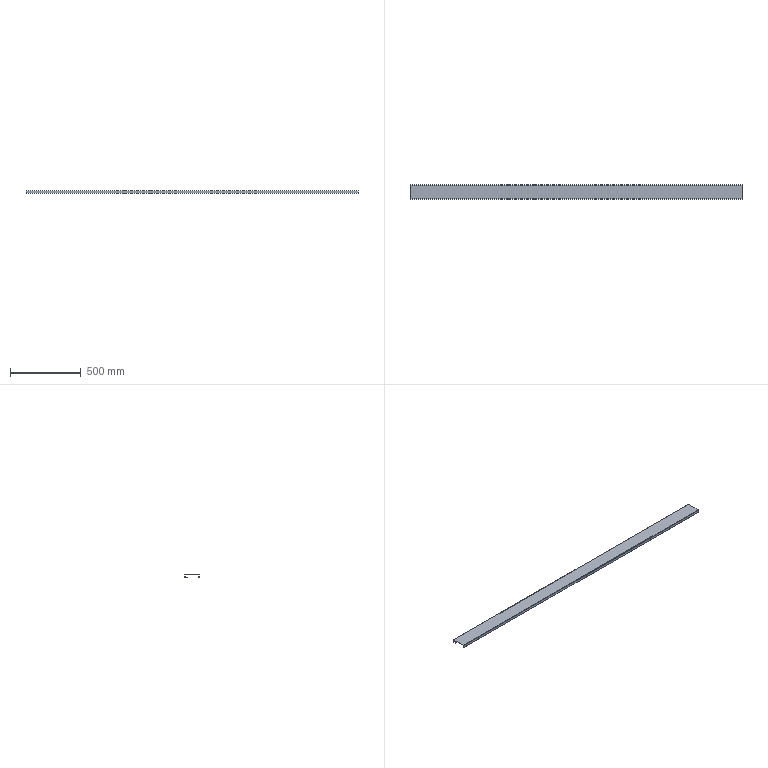Part | STEP file | E3-中转釜护栏8踢脚Plate | 1 solid | 18 faces | box 2340 x 100 x 20 mm | volume 537896 mm3 | plane 12 | cylinder 6 | commonest cylinder face diameters 2 x3 5 x3
STEP:
#1=CARTESIAN_POINT('',(0.,0.,0.));
#2=DIRECTION('',(0.,0.,1.));
#3=DIRECTION('',(1.,0.,0.));
#4=AXIS2_PLACEMENT_3D('',#1,#2,#3);
#5=CARTESIAN_POINT('',(-1170.,1.5,-2.5));
#6=VERTEX_POINT('',#5);
#7=CARTESIAN_POINT('',(-1170.,1.5,-20.));
#8=VERTEX_POINT('',#7);
#9=CARTESIAN_POINT('',(-1170.,1.5,-2.5));
#10=DIRECTION('',(0.,0.,-1.));
#11=VECTOR('',#10,1.);
#12=LINE('',#9,#11);
#13=CARTESIAN_POINT('',(1170.,1.5,-2.5));
#14=DIRECTION('',(0.,-1.,0.));
#15=DIRECTION('',(0.,0.,1.));
#16=AXIS2_PLACEMENT_3D('',#13,#14,#15);
#17=PLANE('',#16);
#18=CARTESIAN_POINT('',(0.,2340.));
#19=DIRECTION('',(-1.,0.));
#20=VECTOR('',#19,1.);
#21=LINE('',#18,#20);
#22=(GEOMETRIC_REPRESENTATION_CONTEXT(2)PARAMETRIC_REPRESENTATION_CONTEXT()REPRESENTATION_CONTEXT('',''));
#23=DEFINITIONAL_REPRESENTATION('',(#21),#22);
#24=PCURVE('',#17,#23);
#25=CARTESIAN_POINT('',(-1170.,2.5,-2.5));
#26=DIRECTION('',(-1.,0.,0.));
#27=DIRECTION('',(0.,0.,-1.));
#28=AXIS2_PLACEMENT_3D('',#25,#26,#27);
#29=PLANE('',#28);
#30=CARTESIAN_POINT('',(0.,1.));
#31=DIRECTION('',(1.,0.));
#32=VECTOR('',#31,1.);
#33=LINE('',#30,#32);
#34=(GEOMETRIC_REPRESENTATION_CONTEXT(2)PARAMETRIC_REPRESENTATION_CONTEXT()REPRESENTATION_CONTEXT('',''));
#35=DEFINITIONAL_REPRESENTATION('',(#33),#34);
#36=PCURVE('',#29,#35);
#37=SURFACE_CURVE('',#12,(#24,#36),.PCURVE_S1.);
#38=EDGE_CURVE('',#6,#8,#37,.T.);
#39=ORIENTED_EDGE('',*,*,#38,.F.);
#40=CARTESIAN_POINT('',(1170.,1.5,-2.5));
#41=VERTEX_POINT('',#40);
#42=CARTESIAN_POINT('',(1170.,1.5,-2.5));
#43=DIRECTION('',(-1.,0.,0.));
#44=VECTOR('',#43,1.);
#45=LINE('',#42,#44);
#46=CARTESIAN_POINT('',(0.,0.));
#47=DIRECTION('',(0.,1.));
#48=VECTOR('',#47,1.);
#49=LINE('',#46,#48);
#50=(GEOMETRIC_REPRESENTATION_CONTEXT(2)PARAMETRIC_REPRESENTATION_CONTEXT()REPRESENTATION_CONTEXT('',''));
#51=DEFINITIONAL_REPRESENTATION('',(#49),#50);
#52=PCURVE('',#17,#51);
#53=CARTESIAN_POINT('',(1170.,2.5,-2.5));
#54=DIRECTION('',(-1.,0.,0.));
#55=DIRECTION('',(0.,0.,-1.));
#56=AXIS2_PLACEMENT_3D('',#53,#54,#55);
#57=CYLINDRICAL_SURFACE('',#56,1.);
#58=CARTESIAN_POINT('',(1.571,0.));
#59=DIRECTION('',(0.,1.));
#60=VECTOR('',#59,1.);
#61=LINE('',#58,#60);
#62=(GEOMETRIC_REPRESENTATION_CONTEXT(2)PARAMETRIC_REPRESENTATION_CONTEXT()REPRESENTATION_CONTEXT('',''));
#63=DEFINITIONAL_REPRESENTATION('',(#61),#62);
#64=PCURVE('',#57,#63);
#65=SURFACE_CURVE('',#45,(#52,#64),.PCURVE_S1.);
#66=EDGE_CURVE('',#41,#6,#65,.T.);
#67=ORIENTED_EDGE('',*,*,#66,.F.);
#68=CARTESIAN_POINT('',(1170.,1.5,-20.));
#69=VERTEX_POINT('',#68);
#70=CARTESIAN_POINT('',(1170.,1.5,-2.5));
#71=DIRECTION('',(0.,0.,-1.));
#72=VECTOR('',#71,1.);
#73=LINE('',#70,#72);
#74=CARTESIAN_POINT('',(0.,0.));
#75=DIRECTION('',(-1.,0.));
#76=VECTOR('',#75,1.);
#77=LINE('',#74,#76);
#78=(GEOMETRIC_REPRESENTATION_CONTEXT(2)PARAMETRIC_REPRESENTATION_CONTEXT()REPRESENTATION_CONTEXT('',''));
#79=DEFINITIONAL_REPRESENTATION('',(#77),#78);
#80=PCURVE('',#17,#79);
#81=CARTESIAN_POINT('',(1170.,2.5,-2.5));
#82=DIRECTION('',(-1.,0.,0.));
#83=DIRECTION('',(0.,0.,-1.));
#84=AXIS2_PLACEMENT_3D('',#81,#82,#83);
#85=PLANE('',#84);
#86=CARTESIAN_POINT('',(0.,1.));
#87=DIRECTION('',(1.,0.));
#88=VECTOR('',#87,1.);
#89=LINE('',#86,#88);
#90=(GEOMETRIC_REPRESENTATION_CONTEXT(2)PARAMETRIC_REPRESENTATION_CONTEXT()REPRESENTATION_CONTEXT('',''));
#91=DEFINITIONAL_REPRESENTATION('',(#89),#90);
#92=PCURVE('',#85,#91);
#93=SURFACE_CURVE('',#73,(#80,#92),.PCURVE_S1.);
#94=EDGE_CURVE('',#41,#69,#93,.T.);
#95=ORIENTED_EDGE('',*,*,#94,.T.);
#96=CARTESIAN_POINT('',(1170.,1.5,-20.));
#97=DIRECTION('',(-1.,0.,0.));
#98=VECTOR('',#97,1.);
#99=LINE('',#96,#98);
#100=CARTESIAN_POINT('',(-17.5,0.));
#101=DIRECTION('',(0.,1.));
#102=VECTOR('',#101,1.);
#103=LINE('',#100,#102);
#104=(GEOMETRIC_REPRESENTATION_CONTEXT(2)PARAMETRIC_REPRESENTATION_CONTEXT()REPRESENTATION_CONTEXT('',''));
#105=DEFINITIONAL_REPRESENTATION('',(#103),#104);
#106=PCURVE('',#17,#105);
#107=CARTESIAN_POINT('',(1170.,0.,-20.));
#108=DIRECTION('',(0.,0.,-1.));
#109=DIRECTION('',(1.,0.,0.));
#110=AXIS2_PLACEMENT_3D('',#107,#108,#109);
#111=PLANE('',#110);
#112=CARTESIAN_POINT('',(0.,-1.5));
#113=DIRECTION('',(-1.,0.));
#114=VECTOR('',#113,1.);
#115=LINE('',#112,#114);
#116=(GEOMETRIC_REPRESENTATION_CONTEXT(2)PARAMETRIC_REPRESENTATION_CONTEXT()REPRESENTATION_CONTEXT('',''));
#117=DEFINITIONAL_REPRESENTATION('',(#115),#116);
#118=PCURVE('',#111,#117);
#119=SURFACE_CURVE('',#99,(#106,#118),.PCURVE_S1.);
#120=EDGE_CURVE('',#69,#8,#119,.T.);
#121=ORIENTED_EDGE('',*,*,#120,.T.);
#122=EDGE_LOOP('',(#39,#67,#95,#121));
#123=FACE_BOUND('',#122,.T.);
#124=ADVANCED_FACE('',(#123),#17,.F.);
#125=CARTESIAN_POINT('',(-1170.,0.,-20.));
#126=VERTEX_POINT('',#125);
#127=CARTESIAN_POINT('',(-1170.,0.,-20.));
#128=DIRECTION('',(0.,1.,0.));
#129=VECTOR('',#128,1.);
#130=LINE('',#127,#129);
#131=CARTESIAN_POINT('',(-2340.,0.));
#132=DIRECTION('',(0.,-1.));
#133=VECTOR('',#132,1.);
#134=LINE('',#131,#133);
#135=(GEOMETRIC_REPRESENTATION_CONTEXT(2)PARAMETRIC_REPRESENTATION_CONTEXT()REPRESENTATION_CONTEXT('',''));
#136=DEFINITIONAL_REPRESENTATION('',(#134),#135);
#137=PCURVE('',#111,#136);
#138=CARTESIAN_POINT('',(17.5,2.5));
#139=DIRECTION('',(0.,-1.));
#140=VECTOR('',#139,1.);
#141=LINE('',#138,#140);
#142=(GEOMETRIC_REPRESENTATION_CONTEXT(2)PARAMETRIC_REPRESENTATION_CONTEXT()REPRESENTATION_CONTEXT('',''));
#143=DEFINITIONAL_REPRESENTATION('',(#141),#142);
#144=PCURVE('',#29,#143);
#145=SURFACE_CURVE('',#130,(#137,#144),.PCURVE_S1.);
#146=EDGE_CURVE('',#126,#8,#145,.T.);
#147=ORIENTED_EDGE('',*,*,#146,.T.);
#148=ORIENTED_EDGE('',*,*,#120,.F.);
#149=CARTESIAN_POINT('',(1170.,0.,-20.));
#150=VERTEX_POINT('',#149);
#151=CARTESIAN_POINT('',(1170.,0.,-20.));
#152=DIRECTION('',(0.,1.,0.));
#153=VECTOR('',#152,1.);
#154=LINE('',#151,#153);
#155=CARTESIAN_POINT('',(0.,0.));
#156=DIRECTION('',(0.,-1.));
#157=VECTOR('',#156,1.);
#158=LINE('',#155,#157);
#159=(GEOMETRIC_REPRESENTATION_CONTEXT(2)PARAMETRIC_REPRESENTATION_CONTEXT()REPRESENTATION_CONTEXT('',''));
#160=DEFINITIONAL_REPRESENTATION('',(#158),#159);
#161=PCURVE('',#111,#160);
#162=CARTESIAN_POINT('',(17.5,2.5));
#163=DIRECTION('',(0.,-1.));
#164=VECTOR('',#163,1.);
#165=LINE('',#162,#164);
#166=(GEOMETRIC_REPRESENTATION_CONTEXT(2)PARAMETRIC_REPRESENTATION_CONTEXT()REPRESENTATION_CONTEXT('',''));
#167=DEFINITIONAL_REPRESENTATION('',(#165),#166);
#168=PCURVE('',#85,#167);
#169=SURFACE_CURVE('',#154,(#161,#168),.PCURVE_S1.);
#170=EDGE_CURVE('',#150,#69,#169,.T.);
#171=ORIENTED_EDGE('',*,*,#170,.F.);
#172=CARTESIAN_POINT('',(1170.,0.,-20.));
#173=DIRECTION('',(-1.,0.,0.));
#174=VECTOR('',#173,1.);
#175=LINE('',#172,#174);
#176=CARTESIAN_POINT('',(0.,0.));
#177=DIRECTION('',(-1.,0.));
#178=VECTOR('',#177,1.);
#179=LINE('',#176,#178);
#180=(GEOMETRIC_REPRESENTATION_CONTEXT(2)PARAMETRIC_REPRESENTATION_CONTEXT()REPRESENTATION_CONTEXT('',''));
#181=DEFINITIONAL_REPRESENTATION('',(#179),#180);
#182=PCURVE('',#111,#181);
#183=CARTESIAN_POINT('',(1170.,0.,-2.5));
#184=DIRECTION('',(0.,-1.,0.));
#185=DIRECTION('',(0.,0.,1.));
#186=AXIS2_PLACEMENT_3D('',#183,#184,#185);
#187=PLANE('',#186);
#188=CARTESIAN_POINT('',(-17.5,0.));
#189=DIRECTION('',(0.,1.));
#190=VECTOR('',#189,1.);
#191=LINE('',#188,#190);
#192=(GEOMETRIC_REPRESENTATION_CONTEXT(2)PARAMETRIC_REPRESENTATION_CONTEXT()REPRESENTATION_CONTEXT('',''));
#193=DEFINITIONAL_REPRESENTATION('',(#191),#192);
#194=PCURVE('',#187,#193);
#195=SURFACE_CURVE('',#175,(#182,#194),.PCURVE_S1.);
#196=EDGE_CURVE('',#150,#126,#195,.T.);
#197=ORIENTED_EDGE('',*,*,#196,.T.);
#198=EDGE_LOOP('',(#147,#148,#171,#197));
#199=FACE_BOUND('',#198,.T.);
#200=ADVANCED_FACE('',(#199),#111,.T.);
#201=CARTESIAN_POINT('',(-1170.,0.,-2.5));
#202=VERTEX_POINT('',#201);
#203=CARTESIAN_POINT('',(-1170.,0.,-2.5));
#204=DIRECTION('',(0.,0.,-1.));
#205=VECTOR('',#204,1.);
#206=LINE('',#203,#205);
#207=CARTESIAN_POINT('',(0.,2340.));
#208=DIRECTION('',(-1.,0.));
#209=VECTOR('',#208,1.);
#210=LINE('',#207,#209);
#211=(GEOMETRIC_REPRESENTATION_CONTEXT(2)PARAMETRIC_REPRESENTATION_CONTEXT()REPRESENTATION_CONTEXT('',''));
#212=DEFINITIONAL_REPRESENTATION('',(#210),#211);
#213=PCURVE('',#187,#212);
#214=CARTESIAN_POINT('',(0.,2.5));
#215=DIRECTION('',(1.,0.));
#216=VECTOR('',#215,1.);
#217=LINE('',#214,#216);
#218=(GEOMETRIC_REPRESENTATION_CONTEXT(2)PARAMETRIC_REPRESENTATION_CONTEXT()REPRESENTATION_CONTEXT('',''));
#219=DEFINITIONAL_REPRESENTATION('',(#217),#218);
#220=PCURVE('',#29,#219);
#221=SURFACE_CURVE('',#206,(#213,#220),.PCURVE_S1.);
#222=EDGE_CURVE('',#202,#126,#221,.T.);
#223=ORIENTED_EDGE('',*,*,#222,.T.);
#224=ORIENTED_EDGE('',*,*,#196,.F.);
#225=CARTESIAN_POINT('',(1170.,0.,-2.5));
#226=VERTEX_POINT('',#225);
#227=CARTESIAN_POINT('',(1170.,0.,-2.5));
#228=DIRECTION('',(0.,0.,-1.));
#229=VECTOR('',#228,1.);
#230=LINE('',#227,#229);
#231=CARTESIAN_POINT('',(0.,0.));
#232=DIRECTION('',(-1.,0.));
#233=VECTOR('',#232,1.);
#234=LINE('',#231,#233);
#235=(GEOMETRIC_REPRESENTATION_CONTEXT(2)PARAMETRIC_REPRESENTATION_CONTEXT()REPRESENTATION_CONTEXT('',''));
#236=DEFINITIONAL_REPRESENTATION('',(#234),#235);
#237=PCURVE('',#187,#236);
#238=CARTESIAN_POINT('',(0.,2.5));
#239=DIRECTION('',(1.,0.));
#240=VECTOR('',#239,1.);
#241=LINE('',#238,#240);
#242=(GEOMETRIC_REPRESENTATION_CONTEXT(2)PARAMETRIC_REPRESENTATION_CONTEXT()REPRESENTATION_CONTEXT('',''));
#243=DEFINITIONAL_REPRESENTATION('',(#241),#242);
#244=PCURVE('',#85,#243);
#245=SURFACE_CURVE('',#230,(#237,#244),.PCURVE_S1.);
#246=EDGE_CURVE('',#226,#150,#245,.T.);
#247=ORIENTED_EDGE('',*,*,#246,.F.);
#248=CARTESIAN_POINT('',(1170.,0.,-2.5));
#249=DIRECTION('',(-1.,0.,0.));
#250=VECTOR('',#249,1.);
#251=LINE('',#248,#250);
#252=CARTESIAN_POINT('',(0.,0.));
#253=DIRECTION('',(0.,1.));
#254=VECTOR('',#253,1.);
#255=LINE('',#252,#254);
#256=(GEOMETRIC_REPRESENTATION_CONTEXT(2)PARAMETRIC_REPRESENTATION_CONTEXT()REPRESENTATION_CONTEXT('',''));
#257=DEFINITIONAL_REPRESENTATION('',(#255),#256);
#258=PCURVE('',#187,#257);
#259=CARTESIAN_POINT('',(1170.,2.5,-2.5));
#260=DIRECTION('',(-1.,0.,0.));
#261=DIRECTION('',(0.,0.,-1.));
#262=AXIS2_PLACEMENT_3D('',#259,#260,#261);
#263=CYLINDRICAL_SURFACE('',#262,2.5);
#264=CARTESIAN_POINT('',(1.571,0.));
#265=DIRECTION('',(0.,1.));
#266=VECTOR('',#265,1.);
#267=LINE('',#264,#266);
#268=(GEOMETRIC_REPRESENTATION_CONTEXT(2)PARAMETRIC_REPRESENTATION_CONTEXT()REPRESENTATION_CONTEXT('',''));
#269=DEFINITIONAL_REPRESENTATION('',(#267),#268);
#270=PCURVE('',#263,#269);
#271=SURFACE_CURVE('',#251,(#258,#270),.PCURVE_S1.);
#272=EDGE_CURVE('',#226,#202,#271,.T.);
#273=ORIENTED_EDGE('',*,*,#272,.T.);
#274=EDGE_LOOP('',(#223,#224,#247,#273));
#275=FACE_BOUND('',#274,.T.);
#276=ADVANCED_FACE('',(#275),#187,.T.);
#277=CARTESIAN_POINT('',(-1170.,2.5,0.));
#278=VERTEX_POINT('',#277);
#279=CARTESIAN_POINT('',(-1170.,2.5,-2.5));
#280=DIRECTION('',(1.,0.,0.));
#281=DIRECTION('',(0.,0.,-1.));
#282=AXIS2_PLACEMENT_3D('',#279,#280,#281);
#283=CIRCLE('',#282,2.5);
#284=CARTESIAN_POINT('',(6.283,2340.));
#285=DIRECTION('',(-1.,0.));
#286=VECTOR('',#285,1.);
#287=LINE('',#284,#286);
#288=(GEOMETRIC_REPRESENTATION_CONTEXT(2)PARAMETRIC_REPRESENTATION_CONTEXT()REPRESENTATION_CONTEXT('',''));
#289=DEFINITIONAL_REPRESENTATION('',(#287),#288);
#290=PCURVE('',#263,#289);
#291=CARTESIAN_POINT('',(2.5,0.));
#292=CARTESIAN_POINT('',(2.5,-4.33));
#293=CARTESIAN_POINT('',(-1.25,-2.165));
#294=CARTESIAN_POINT('',(-5.,0.));
#295=CARTESIAN_POINT('',(-1.25,2.165));
#296=CARTESIAN_POINT('',(2.5,4.33));
#297=CARTESIAN_POINT('',(2.5,0.));
#298=(BOUNDED_CURVE()B_SPLINE_CURVE(2,(#291,#292,#293,#294,#295,#296,#297),.UNSPECIFIED.,.T.,.F.)B_SPLINE_CURVE_WITH_KNOTS((1,2,2,2,2,1),(-2.094,0.,2.094,4.189,6.283,8.378),.UNSPECIFIED.)CURVE()GEOMETRIC_REPRESENTATION_ITEM()RATIONAL_B_SPLINE_CURVE((1.,0.5,1.,0.5,1.,0.5,1.))REPRESENTATION_ITEM(''));
#299=(GEOMETRIC_REPRESENTATION_CONTEXT(2)PARAMETRIC_REPRESENTATION_CONTEXT()REPRESENTATION_CONTEXT('',''));
#300=DEFINITIONAL_REPRESENTATION('',(#298),#299);
#301=PCURVE('',#29,#300);
#302=SURFACE_CURVE('',#283,(#290,#301),.PCURVE_S1.);
#303=EDGE_CURVE('',#278,#202,#302,.T.);
#304=ORIENTED_EDGE('',*,*,#303,.T.);
#305=ORIENTED_EDGE('',*,*,#272,.F.);
#306=CARTESIAN_POINT('',(1170.,2.5,0.));
#307=VERTEX_POINT('',#306);
#308=CARTESIAN_POINT('',(1170.,2.5,-2.5));
#309=DIRECTION('',(1.,0.,0.));
#310=DIRECTION('',(0.,0.,-1.));
#311=AXIS2_PLACEMENT_3D('',#308,#309,#310);
#312=CIRCLE('',#311,2.5);
#313=CARTESIAN_POINT('',(6.283,0.));
#314=DIRECTION('',(-1.,0.));
#315=VECTOR('',#314,1.);
#316=LINE('',#313,#315);
#317=(GEOMETRIC_REPRESENTATION_CONTEXT(2)PARAMETRIC_REPRESENTATION_CONTEXT()REPRESENTATION_CONTEXT('',''));
#318=DEFINITIONAL_REPRESENTATION('',(#316),#317);
#319=PCURVE('',#263,#318);
#320=CARTESIAN_POINT('',(2.5,0.));
#321=CARTESIAN_POINT('',(2.5,-4.33));
#322=CARTESIAN_POINT('',(-1.25,-2.165));
#323=CARTESIAN_POINT('',(-5.,0.));
#324=CARTESIAN_POINT('',(-1.25,2.165));
#325=CARTESIAN_POINT('',(2.5,4.33));
#326=CARTESIAN_POINT('',(2.5,0.));
#327=(BOUNDED_CURVE()B_SPLINE_CURVE(2,(#320,#321,#322,#323,#324,#325,#326),.UNSPECIFIED.,.T.,.F.)B_SPLINE_CURVE_WITH_KNOTS((1,2,2,2,2,1),(-2.094,0.,2.094,4.189,6.283,8.378),.UNSPECIFIED.)CURVE()GEOMETRIC_REPRESENTATION_ITEM()RATIONAL_B_SPLINE_CURVE((1.,0.5,1.,0.5,1.,0.5,1.))REPRESENTATION_ITEM(''));
#328=(GEOMETRIC_REPRESENTATION_CONTEXT(2)PARAMETRIC_REPRESENTATION_CONTEXT()REPRESENTATION_CONTEXT('',''));
#329=DEFINITIONAL_REPRESENTATION('',(#327),#328);
#330=PCURVE('',#85,#329);
#331=SURFACE_CURVE('',#312,(#319,#330),.PCURVE_S1.);
#332=EDGE_CURVE('',#307,#226,#331,.T.);
#333=ORIENTED_EDGE('',*,*,#332,.F.);
#334=CARTESIAN_POINT('',(1170.,2.5,0.));
#335=DIRECTION('',(-1.,0.,0.));
#336=VECTOR('',#335,1.);
#337=LINE('',#334,#336);
#338=CARTESIAN_POINT('',(3.142,0.));
#339=DIRECTION('',(0.,1.));
#340=VECTOR('',#339,1.);
#341=LINE('',#338,#340);
#342=(GEOMETRIC_REPRESENTATION_CONTEXT(2)PARAMETRIC_REPRESENTATION_CONTEXT()REPRESENTATION_CONTEXT('',''));
#343=DEFINITIONAL_REPRESENTATION('',(#341),#342);
#344=PCURVE('',#263,#343);
#345=CARTESIAN_POINT('',(1170.,2.5,0.));
#346=DIRECTION('',(0.,0.,1.));
#347=DIRECTION('',(-1.,0.,0.));
#348=AXIS2_PLACEMENT_3D('',#345,#346,#347);
#349=PLANE('',#348);
#350=CARTESIAN_POINT('',(0.,0.));
#351=DIRECTION('',(1.,0.));
#352=VECTOR('',#351,1.);
#353=LINE('',#350,#352);
#354=(GEOMETRIC_REPRESENTATION_CONTEXT(2)PARAMETRIC_REPRESENTATION_CONTEXT()REPRESENTATION_CONTEXT('',''));
#355=DEFINITIONAL_REPRESENTATION('',(#353),#354);
#356=PCURVE('',#349,#355);
#357=SURFACE_CURVE('',#337,(#344,#356),.PCURVE_S1.);
#358=EDGE_CURVE('',#307,#278,#357,.T.);
#359=ORIENTED_EDGE('',*,*,#358,.T.);
#360=EDGE_LOOP('',(#304,#305,#333,#359));
#361=FACE_BOUND('',#360,.T.);
#362=ADVANCED_FACE('',(#361),#263,.T.);
#363=CARTESIAN_POINT('',(-1170.,97.5,0.));
#364=VERTEX_POINT('',#363);
#365=CARTESIAN_POINT('',(-1170.,2.5,0.));
#366=DIRECTION('',(0.,-1.,0.));
#367=VECTOR('',#366,1.);
#368=LINE('',#365,#367);
#369=CARTESIAN_POINT('',(2340.,0.));
#370=DIRECTION('',(0.,1.));
#371=VECTOR('',#370,1.);
#372=LINE('',#369,#371);
#373=(GEOMETRIC_REPRESENTATION_CONTEXT(2)PARAMETRIC_REPRESENTATION_CONTEXT()REPRESENTATION_CONTEXT('',''));
#374=DEFINITIONAL_REPRESENTATION('',(#372),#373);
#375=PCURVE('',#349,#374);
#376=CARTESIAN_POINT('',(-2.5,0.));
#377=DIRECTION('',(0.,1.));
#378=VECTOR('',#377,1.);
#379=LINE('',#376,#378);
#380=(GEOMETRIC_REPRESENTATION_CONTEXT(2)PARAMETRIC_REPRESENTATION_CONTEXT()REPRESENTATION_CONTEXT('',''));
#381=DEFINITIONAL_REPRESENTATION('',(#379),#380);
#382=PCURVE('',#29,#381);
#383=SURFACE_CURVE('',#368,(#375,#382),.PCURVE_S1.);
#384=EDGE_CURVE('',#364,#278,#383,.T.);
#385=ORIENTED_EDGE('',*,*,#384,.T.);
#386=ORIENTED_EDGE('',*,*,#358,.F.);
#387=CARTESIAN_POINT('',(1170.,97.5,0.));
#388=VERTEX_POINT('',#387);
#389=CARTESIAN_POINT('',(1170.,2.5,0.));
#390=DIRECTION('',(0.,-1.,0.));
#391=VECTOR('',#390,1.);
#392=LINE('',#389,#391);
#393=CARTESIAN_POINT('',(0.,0.));
#394=DIRECTION('',(0.,1.));
#395=VECTOR('',#394,1.);
#396=LINE('',#393,#395);
#397=(GEOMETRIC_REPRESENTATION_CONTEXT(2)PARAMETRIC_REPRESENTATION_CONTEXT()REPRESENTATION_CONTEXT('',''));
#398=DEFINITIONAL_REPRESENTATION('',(#396),#397);
#399=PCURVE('',#349,#398);
#400=CARTESIAN_POINT('',(-2.5,0.));
#401=DIRECTION('',(0.,1.));
#402=VECTOR('',#401,1.);
#403=LINE('',#400,#402);
#404=(GEOMETRIC_REPRESENTATION_CONTEXT(2)PARAMETRIC_REPRESENTATION_CONTEXT()REPRESENTATION_CONTEXT('',''));
#405=DEFINITIONAL_REPRESENTATION('',(#403),#404);
#406=PCURVE('',#85,#405);
#407=SURFACE_CURVE('',#392,(#399,#406),.PCURVE_S1.);
#408=EDGE_CURVE('',#388,#307,#407,.T.);
#409=ORIENTED_EDGE('',*,*,#408,.F.);
#410=CARTESIAN_POINT('',(1170.,97.5,0.));
#411=DIRECTION('',(-1.,0.,0.));
#412=VECTOR('',#411,1.);
#413=LINE('',#410,#412);
#414=CARTESIAN_POINT('',(0.,-95.));
#415=DIRECTION('',(1.,0.));
#416=VECTOR('',#415,1.);
#417=LINE('',#414,#416);
#418=(GEOMETRIC_REPRESENTATION_CONTEXT(2)PARAMETRIC_REPRESENTATION_CONTEXT()REPRESENTATION_CONTEXT('',''));
#419=DEFINITIONAL_REPRESENTATION('',(#417),#418);
#420=PCURVE('',#349,#419);
#421=CARTESIAN_POINT('',(1170.,97.5,-2.5));
#422=DIRECTION('',(-1.,0.,0.));
#423=DIRECTION('',(0.,0.,-1.));
#424=AXIS2_PLACEMENT_3D('',#421,#422,#423);
#425=CYLINDRICAL_SURFACE('',#424,2.5);
#426=CARTESIAN_POINT('',(3.142,0.));
#427=DIRECTION('',(0.,1.));
#428=VECTOR('',#427,1.);
#429=LINE('',#426,#428);
#430=(GEOMETRIC_REPRESENTATION_CONTEXT(2)PARAMETRIC_REPRESENTATION_CONTEXT()REPRESENTATION_CONTEXT('',''));
#431=DEFINITIONAL_REPRESENTATION('',(#429),#430);
#432=PCURVE('',#425,#431);
#433=SURFACE_CURVE('',#413,(#420,#432),.PCURVE_S1.);
#434=EDGE_CURVE('',#388,#364,#433,.T.);
#435=ORIENTED_EDGE('',*,*,#434,.T.);
#436=EDGE_LOOP('',(#385,#386,#409,#435));
#437=FACE_BOUND('',#436,.T.);
#438=ADVANCED_FACE('',(#437),#349,.T.);
#439=CARTESIAN_POINT('',(-1170.,100.,-2.5));
#440=VERTEX_POINT('',#439);
#441=CARTESIAN_POINT('',(-1170.,97.5,-2.5));
#442=DIRECTION('',(1.,0.,0.));
#443=DIRECTION('',(0.,0.,1.));
#444=AXIS2_PLACEMENT_3D('',#441,#442,#443);
#445=CIRCLE('',#444,2.5);
#446=CARTESIAN_POINT('',(9.425,2340.));
#447=DIRECTION('',(-1.,0.));
#448=VECTOR('',#447,1.);
#449=LINE('',#446,#448);
#450=(GEOMETRIC_REPRESENTATION_CONTEXT(2)PARAMETRIC_REPRESENTATION_CONTEXT()REPRESENTATION_CONTEXT('',''));
#451=DEFINITIONAL_REPRESENTATION('',(#449),#450);
#452=PCURVE('',#425,#451);
#453=CARTESIAN_POINT('',(-2.5,-95.));
#454=CARTESIAN_POINT('',(-2.5,-90.67));
#455=CARTESIAN_POINT('',(1.25,-92.835));
#456=CARTESIAN_POINT('',(5.,-95.));
#457=CARTESIAN_POINT('',(1.25,-97.165));
#458=CARTESIAN_POINT('',(-2.5,-99.33));
#459=CARTESIAN_POINT('',(-2.5,-95.));
#460=(BOUNDED_CURVE()B_SPLINE_CURVE(2,(#453,#454,#455,#456,#457,#458,#459),.UNSPECIFIED.,.T.,.F.)B_SPLINE_CURVE_WITH_KNOTS((1,2,2,2,2,1),(-2.094,0.,2.094,4.189,6.283,8.378),.UNSPECIFIED.)CURVE()GEOMETRIC_REPRESENTATION_ITEM()RATIONAL_B_SPLINE_CURVE((1.,0.5,1.,0.5,1.,0.5,1.))REPRESENTATION_ITEM(''));
#461=(GEOMETRIC_REPRESENTATION_CONTEXT(2)PARAMETRIC_REPRESENTATION_CONTEXT()REPRESENTATION_CONTEXT('',''));
#462=DEFINITIONAL_REPRESENTATION('',(#460),#461);
#463=PCURVE('',#29,#462);
#464=SURFACE_CURVE('',#445,(#452,#463),.PCURVE_S1.);
#465=EDGE_CURVE('',#440,#364,#464,.T.);
#466=ORIENTED_EDGE('',*,*,#465,.T.);
#467=ORIENTED_EDGE('',*,*,#434,.F.);
#468=CARTESIAN_POINT('',(1170.,100.,-2.5));
#469=VERTEX_POINT('',#468);
#470=CARTESIAN_POINT('',(1170.,97.5,-2.5));
#471=DIRECTION('',(1.,0.,0.));
#472=DIRECTION('',(0.,0.,1.));
#473=AXIS2_PLACEMENT_3D('',#470,#471,#472);
#474=CIRCLE('',#473,2.5);
#475=CARTESIAN_POINT('',(9.425,0.));
#476=DIRECTION('',(-1.,0.));
#477=VECTOR('',#476,1.);
#478=LINE('',#475,#477);
#479=(GEOMETRIC_REPRESENTATION_CONTEXT(2)PARAMETRIC_REPRESENTATION_CONTEXT()REPRESENTATION_CONTEXT('',''));
#480=DEFINITIONAL_REPRESENTATION('',(#478),#479);
#481=PCURVE('',#425,#480);
#482=CARTESIAN_POINT('',(-2.5,-95.));
#483=CARTESIAN_POINT('',(-2.5,-90.67));
#484=CARTESIAN_POINT('',(1.25,-92.835));
#485=CARTESIAN_POINT('',(5.,-95.));
#486=CARTESIAN_POINT('',(1.25,-97.165));
#487=CARTESIAN_POINT('',(-2.5,-99.33));
#488=CARTESIAN_POINT('',(-2.5,-95.));
#489=(BOUNDED_CURVE()B_SPLINE_CURVE(2,(#482,#483,#484,#485,#486,#487,#488),.UNSPECIFIED.,.T.,.F.)B_SPLINE_CURVE_WITH_KNOTS((1,2,2,2,2,1),(-2.094,0.,2.094,4.189,6.283,8.378),.UNSPECIFIED.)CURVE()GEOMETRIC_REPRESENTATION_ITEM()RATIONAL_B_SPLINE_CURVE((1.,0.5,1.,0.5,1.,0.5,1.))REPRESENTATION_ITEM(''));
#490=(GEOMETRIC_REPRESENTATION_CONTEXT(2)PARAMETRIC_REPRESENTATION_CONTEXT()REPRESENTATION_CONTEXT('',''));
#491=DEFINITIONAL_REPRESENTATION('',(#489),#490);
#492=PCURVE('',#85,#491);
#493=SURFACE_CURVE('',#474,(#481,#492),.PCURVE_S1.);
#494=EDGE_CURVE('',#469,#388,#493,.T.);
#495=ORIENTED_EDGE('',*,*,#494,.F.);
#496=CARTESIAN_POINT('',(1170.,100.,-2.5));
#497=DIRECTION('',(-1.,0.,0.));
#498=VECTOR('',#497,1.);
#499=LINE('',#496,#498);
#500=CARTESIAN_POINT('',(4.712,0.));
#501=DIRECTION('',(0.,1.));
#502=VECTOR('',#501,1.);
#503=LINE('',#500,#502);
#504=(GEOMETRIC_REPRESENTATION_CONTEXT(2)PARAMETRIC_REPRESENTATION_CONTEXT()REPRESENTATION_CONTEXT('',''));
#505=DEFINITIONAL_REPRESENTATION('',(#503),#504);
#506=PCURVE('',#425,#505);
#507=CARTESIAN_POINT('',(1170.,100.,-2.5));
#508=DIRECTION('',(0.,1.,0.));
#509=DIRECTION('',(0.,0.,-1.));
#510=AXIS2_PLACEMENT_3D('',#507,#508,#509);
#511=PLANE('',#510);
#512=CARTESIAN_POINT('',(0.,0.));
#513=DIRECTION('',(0.,1.));
#514=VECTOR('',#513,1.);
#515=LINE('',#512,#514);
#516=(GEOMETRIC_REPRESENTATION_CONTEXT(2)PARAMETRIC_REPRESENTATION_CONTEXT()REPRESENTATION_CONTEXT('',''));
#517=DEFINITIONAL_REPRESENTATION('',(#515),#516);
#518=PCURVE('',#511,#517);
#519=SURFACE_CURVE('',#499,(#506,#518),.PCURVE_S1.);
#520=EDGE_CURVE('',#469,#440,#519,.T.);
#521=ORIENTED_EDGE('',*,*,#520,.T.);
#522=EDGE_LOOP('',(#466,#467,#495,#521));
#523=FACE_BOUND('',#522,.T.);
#524=ADVANCED_FACE('',(#523),#425,.T.);
#525=CARTESIAN_POINT('',(-1170.,100.,-17.5));
#526=VERTEX_POINT('',#525);
#527=CARTESIAN_POINT('',(-1170.,100.,-2.5));
#528=DIRECTION('',(0.,0.,1.));
#529=VECTOR('',#528,1.);
#530=LINE('',#527,#529);
#531=CARTESIAN_POINT('',(0.,2340.));
#532=DIRECTION('',(-1.,0.));
#533=VECTOR('',#532,1.);
#534=LINE('',#531,#533);
#535=(GEOMETRIC_REPRESENTATION_CONTEXT(2)PARAMETRIC_REPRESENTATION_CONTEXT()REPRESENTATION_CONTEXT('',''));
#536=DEFINITIONAL_REPRESENTATION('',(#534),#535);
#537=PCURVE('',#511,#536);
#538=CARTESIAN_POINT('',(0.,-97.5));
#539=DIRECTION('',(-1.,0.));
#540=VECTOR('',#539,1.);
#541=LINE('',#538,#540);
#542=(GEOMETRIC_REPRESENTATION_CONTEXT(2)PARAMETRIC_REPRESENTATION_CONTEXT()REPRESENTATION_CONTEXT('',''));
#543=DEFINITIONAL_REPRESENTATION('',(#541),#542);
#544=PCURVE('',#29,#543);
#545=SURFACE_CURVE('',#530,(#537,#544),.PCURVE_S1.);
#546=EDGE_CURVE('',#526,#440,#545,.T.);
#547=ORIENTED_EDGE('',*,*,#546,.T.);
#548=ORIENTED_EDGE('',*,*,#520,.F.);
#549=CARTESIAN_POINT('',(1170.,100.,-17.5));
#550=VERTEX_POINT('',#549);
#551=CARTESIAN_POINT('',(1170.,100.,-2.5));
#552=DIRECTION('',(0.,0.,1.));
#553=VECTOR('',#552,1.);
#554=LINE('',#551,#553);
#555=CARTESIAN_POINT('',(0.,0.));
#556=DIRECTION('',(-1.,0.));
#557=VECTOR('',#556,1.);
#558=LINE('',#555,#557);
#559=(GEOMETRIC_REPRESENTATION_CONTEXT(2)PARAMETRIC_REPRESENTATION_CONTEXT()REPRESENTATION_CONTEXT('',''));
#560=DEFINITIONAL_REPRESENTATION('',(#558),#559);
#561=PCURVE('',#511,#560);
#562=CARTESIAN_POINT('',(0.,-97.5));
#563=DIRECTION('',(-1.,0.));
#564=VECTOR('',#563,1.);
#565=LINE('',#562,#564);
#566=(GEOMETRIC_REPRESENTATION_CONTEXT(2)PARAMETRIC_REPRESENTATION_CONTEXT()REPRESENTATION_CONTEXT('',''));
#567=DEFINITIONAL_REPRESENTATION('',(#565),#566);
#568=PCURVE('',#85,#567);
#569=SURFACE_CURVE('',#554,(#561,#568),.PCURVE_S1.);
#570=EDGE_CURVE('',#550,#469,#569,.T.);
#571=ORIENTED_EDGE('',*,*,#570,.F.);
#572=CARTESIAN_POINT('',(1170.,100.,-17.5));
#573=DIRECTION('',(-1.,0.,0.));
#574=VECTOR('',#573,1.);
#575=LINE('',#572,#574);
#576=CARTESIAN_POINT('',(15.,0.));
#577=DIRECTION('',(0.,1.));
#578=VECTOR('',#577,1.);
#579=LINE('',#576,#578);
#580=(GEOMETRIC_REPRESENTATION_CONTEXT(2)PARAMETRIC_REPRESENTATION_CONTEXT()REPRESENTATION_CONTEXT('',''));
#581=DEFINITIONAL_REPRESENTATION('',(#579),#580);
#582=PCURVE('',#511,#581);
#583=CARTESIAN_POINT('',(1170.,97.5,-17.5));
#584=DIRECTION('',(-1.,0.,0.));
#585=DIRECTION('',(0.,0.,-1.));
#586=AXIS2_PLACEMENT_3D('',#583,#584,#585);
#587=CYLINDRICAL_SURFACE('',#586,2.5);
#588=CARTESIAN_POINT('',(4.712,0.));
#589=DIRECTION('',(0.,1.));
#590=VECTOR('',#589,1.);
#591=LINE('',#588,#590);
#592=(GEOMETRIC_REPRESENTATION_CONTEXT(2)PARAMETRIC_REPRESENTATION_CONTEXT()REPRESENTATION_CONTEXT('',''));
#593=DEFINITIONAL_REPRESENTATION('',(#591),#592);
#594=PCURVE('',#587,#593);
#595=SURFACE_CURVE('',#575,(#582,#594),.PCURVE_S1.);
#596=EDGE_CURVE('',#550,#526,#595,.T.);
#597=ORIENTED_EDGE('',*,*,#596,.T.);
#598=EDGE_LOOP('',(#547,#548,#571,#597));
#599=FACE_BOUND('',#598,.T.);
#600=ADVANCED_FACE('',(#599),#511,.T.);
#601=CARTESIAN_POINT('',(-1170.,97.5,-20.));
#602=VERTEX_POINT('',#601);
#603=CARTESIAN_POINT('',(-1170.,97.5,-17.5));
#604=DIRECTION('',(1.,0.,0.));
#605=DIRECTION('',(0.,0.,1.));
#606=AXIS2_PLACEMENT_3D('',#603,#604,#605);
#607=CIRCLE('',#606,2.5);
#608=CARTESIAN_POINT('',(9.425,2340.));
#609=DIRECTION('',(-1.,0.));
#610=VECTOR('',#609,1.);
#611=LINE('',#608,#610);
#612=(GEOMETRIC_REPRESENTATION_CONTEXT(2)PARAMETRIC_REPRESENTATION_CONTEXT()REPRESENTATION_CONTEXT('',''));
#613=DEFINITIONAL_REPRESENTATION('',(#611),#612);
#614=PCURVE('',#587,#613);
#615=CARTESIAN_POINT('',(12.5,-95.));
#616=CARTESIAN_POINT('',(12.5,-90.67));
#617=CARTESIAN_POINT('',(16.25,-92.835));
#618=CARTESIAN_POINT('',(20.,-95.));
#619=CARTESIAN_POINT('',(16.25,-97.165));
#620=CARTESIAN_POINT('',(12.5,-99.33));
#621=CARTESIAN_POINT('',(12.5,-95.));
#622=(BOUNDED_CURVE()B_SPLINE_CURVE(2,(#615,#616,#617,#618,#619,#620,#621),.UNSPECIFIED.,.T.,.F.)B_SPLINE_CURVE_WITH_KNOTS((1,2,2,2,2,1),(-2.094,0.,2.094,4.189,6.283,8.378),.UNSPECIFIED.)CURVE()GEOMETRIC_REPRESENTATION_ITEM()RATIONAL_B_SPLINE_CURVE((1.,0.5,1.,0.5,1.,0.5,1.))REPRESENTATION_ITEM(''));
#623=(GEOMETRIC_REPRESENTATION_CONTEXT(2)PARAMETRIC_REPRESENTATION_CONTEXT()REPRESENTATION_CONTEXT('',''));
#624=DEFINITIONAL_REPRESENTATION('',(#622),#623);
#625=PCURVE('',#29,#624);
#626=SURFACE_CURVE('',#607,(#614,#625),.PCURVE_S1.);
#627=EDGE_CURVE('',#602,#526,#626,.T.);
#628=ORIENTED_EDGE('',*,*,#627,.T.);
#629=ORIENTED_EDGE('',*,*,#596,.F.);
#630=CARTESIAN_POINT('',(1170.,97.5,-20.));
#631=VERTEX_POINT('',#630);
#632=CARTESIAN_POINT('',(1170.,97.5,-17.5));
#633=DIRECTION('',(1.,0.,0.));
#634=DIRECTION('',(0.,0.,1.));
#635=AXIS2_PLACEMENT_3D('',#632,#633,#634);
#636=CIRCLE('',#635,2.5);
#637=CARTESIAN_POINT('',(9.425,0.));
#638=DIRECTION('',(-1.,0.));
#639=VECTOR('',#638,1.);
#640=LINE('',#637,#639);
#641=(GEOMETRIC_REPRESENTATION_CONTEXT(2)PARAMETRIC_REPRESENTATION_CONTEXT()REPRESENTATION_CONTEXT('',''));
#642=DEFINITIONAL_REPRESENTATION('',(#640),#641);
#643=PCURVE('',#587,#642);
#644=CARTESIAN_POINT('',(12.5,-95.));
#645=CARTESIAN_POINT('',(12.5,-90.67));
#646=CARTESIAN_POINT('',(16.25,-92.835));
#647=CARTESIAN_POINT('',(20.,-95.));
#648=CARTESIAN_POINT('',(16.25,-97.165));
#649=CARTESIAN_POINT('',(12.5,-99.33));
#650=CARTESIAN_POINT('',(12.5,-95.));
#651=(BOUNDED_CURVE()B_SPLINE_CURVE(2,(#644,#645,#646,#647,#648,#649,#650),.UNSPECIFIED.,.T.,.F.)B_SPLINE_CURVE_WITH_KNOTS((1,2,2,2,2,1),(-2.094,0.,2.094,4.189,6.283,8.378),.UNSPECIFIED.)CURVE()GEOMETRIC_REPRESENTATION_ITEM()RATIONAL_B_SPLINE_CURVE((1.,0.5,1.,0.5,1.,0.5,1.))REPRESENTATION_ITEM(''));
#652=(GEOMETRIC_REPRESENTATION_CONTEXT(2)PARAMETRIC_REPRESENTATION_CONTEXT()REPRESENTATION_CONTEXT('',''));
#653=DEFINITIONAL_REPRESENTATION('',(#651),#652);
#654=PCURVE('',#85,#653);
#655=SURFACE_CURVE('',#636,(#643,#654),.PCURVE_S1.);
#656=EDGE_CURVE('',#631,#550,#655,.T.);
#657=ORIENTED_EDGE('',*,*,#656,.F.);
#658=CARTESIAN_POINT('',(1170.,97.5,-20.));
#659=DIRECTION('',(-1.,0.,0.));
#660=VECTOR('',#659,1.);
#661=LINE('',#658,#660);
#662=CARTESIAN_POINT('',(6.283,0.));
#663=DIRECTION('',(0.,1.));
#664=VECTOR('',#663,1.);
#665=LINE('',#662,#664);
#666=(GEOMETRIC_REPRESENTATION_CONTEXT(2)PARAMETRIC_REPRESENTATION_CONTEXT()REPRESENTATION_CONTEXT('',''));
#667=DEFINITIONAL_REPRESENTATION('',(#665),#666);
#668=PCURVE('',#587,#667);
#669=CARTESIAN_POINT('',(1170.,97.5,-20.));
#670=DIRECTION('',(0.,0.,-1.));
#671=DIRECTION('',(1.,0.,0.));
#672=AXIS2_PLACEMENT_3D('',#669,#670,#671);
#673=PLANE('',#672);
#674=CARTESIAN_POINT('',(0.,0.));
#675=DIRECTION('',(-1.,0.));
#676=VECTOR('',#675,1.);
#677=LINE('',#674,#676);
#678=(GEOMETRIC_REPRESENTATION_CONTEXT(2)PARAMETRIC_REPRESENTATION_CONTEXT()REPRESENTATION_CONTEXT('',''));
#679=DEFINITIONAL_REPRESENTATION('',(#677),#678);
#680=PCURVE('',#673,#679);
#681=SURFACE_CURVE('',#661,(#668,#680),.PCURVE_S1.);
#682=EDGE_CURVE('',#631,#602,#681,.T.);
#683=ORIENTED_EDGE('',*,*,#682,.T.);
#684=EDGE_LOOP('',(#628,#629,#657,#683));
#685=FACE_BOUND('',#684,.T.);
#686=ADVANCED_FACE('',(#685),#587,.T.);
#687=CARTESIAN_POINT('',(-1170.,80.,-20.));
#688=VERTEX_POINT('',#687);
#689=CARTESIAN_POINT('',(-1170.,97.5,-20.));
#690=DIRECTION('',(0.,1.,0.));
#691=VECTOR('',#690,1.);
#692=LINE('',#689,#691);
#693=CARTESIAN_POINT('',(-2340.,0.));
#694=DIRECTION('',(0.,-1.));
#695=VECTOR('',#694,1.);
#696=LINE('',#693,#695);
#697=(GEOMETRIC_REPRESENTATION_CONTEXT(2)PARAMETRIC_REPRESENTATION_CONTEXT()REPRESENTATION_CONTEXT('',''));
#698=DEFINITIONAL_REPRESENTATION('',(#696),#697);
#699=PCURVE('',#673,#698);
#700=CARTESIAN_POINT('',(17.5,-95.));
#701=DIRECTION('',(0.,-1.));
#702=VECTOR('',#701,1.);
#703=LINE('',#700,#702);
#704=(GEOMETRIC_REPRESENTATION_CONTEXT(2)PARAMETRIC_REPRESENTATION_CONTEXT()REPRESENTATION_CONTEXT('',''));
#705=DEFINITIONAL_REPRESENTATION('',(#703),#704);
#706=PCURVE('',#29,#705);
#707=SURFACE_CURVE('',#692,(#699,#706),.PCURVE_S1.);
#708=EDGE_CURVE('',#688,#602,#707,.T.);
#709=ORIENTED_EDGE('',*,*,#708,.T.);
#710=ORIENTED_EDGE('',*,*,#682,.F.);
#711=CARTESIAN_POINT('',(1170.,80.,-20.));
#712=VERTEX_POINT('',#711);
#713=CARTESIAN_POINT('',(1170.,97.5,-20.));
#714=DIRECTION('',(0.,1.,0.));
#715=VECTOR('',#714,1.);
#716=LINE('',#713,#715);
#717=CARTESIAN_POINT('',(0.,0.));
#718=DIRECTION('',(0.,-1.));
#719=VECTOR('',#718,1.);
#720=LINE('',#717,#719);
#721=(GEOMETRIC_REPRESENTATION_CONTEXT(2)PARAMETRIC_REPRESENTATION_CONTEXT()REPRESENTATION_CONTEXT('',''));
#722=DEFINITIONAL_REPRESENTATION('',(#720),#721);
#723=PCURVE('',#673,#722);
#724=CARTESIAN_POINT('',(17.5,-95.));
#725=DIRECTION('',(0.,-1.));
#726=VECTOR('',#725,1.);
#727=LINE('',#724,#726);
#728=(GEOMETRIC_REPRESENTATION_CONTEXT(2)PARAMETRIC_REPRESENTATION_CONTEXT()REPRESENTATION_CONTEXT('',''));
#729=DEFINITIONAL_REPRESENTATION('',(#727),#728);
#730=PCURVE('',#85,#729);
#731=SURFACE_CURVE('',#716,(#723,#730),.PCURVE_S1.);
#732=EDGE_CURVE('',#712,#631,#731,.T.);
#733=ORIENTED_EDGE('',*,*,#732,.F.);
#734=CARTESIAN_POINT('',(1170.,80.,-20.));
#735=DIRECTION('',(-1.,0.,0.));
#736=VECTOR('',#735,1.);
#737=LINE('',#734,#736);
#738=CARTESIAN_POINT('',(0.,17.5));
#739=DIRECTION('',(-1.,0.));
#740=VECTOR('',#739,1.);
#741=LINE('',#738,#740);
#742=(GEOMETRIC_REPRESENTATION_CONTEXT(2)PARAMETRIC_REPRESENTATION_CONTEXT()REPRESENTATION_CONTEXT('',''));
#743=DEFINITIONAL_REPRESENTATION('',(#741),#742);
#744=PCURVE('',#673,#743);
#745=CARTESIAN_POINT('',(1170.,80.,-18.5));
#746=DIRECTION('',(0.,-1.,0.));
#747=DIRECTION('',(0.,0.,1.));
#748=AXIS2_PLACEMENT_3D('',#745,#746,#747);
#749=PLANE('',#748);
#750=CARTESIAN_POINT('',(-1.5,0.));
#751=DIRECTION('',(0.,1.));
#752=VECTOR('',#751,1.);
#753=LINE('',#750,#752);
#754=(GEOMETRIC_REPRESENTATION_CONTEXT(2)PARAMETRIC_REPRESENTATION_CONTEXT()REPRESENTATION_CONTEXT('',''));
#755=DEFINITIONAL_REPRESENTATION('',(#753),#754);
#756=PCURVE('',#749,#755);
#757=SURFACE_CURVE('',#737,(#744,#756),.PCURVE_S1.);
#758=EDGE_CURVE('',#712,#688,#757,.T.);
#759=ORIENTED_EDGE('',*,*,#758,.T.);
#760=EDGE_LOOP('',(#709,#710,#733,#759));
#761=FACE_BOUND('',#760,.T.);
#762=ADVANCED_FACE('',(#761),#673,.T.);
#763=CARTESIAN_POINT('',(-1170.,80.,-18.5));
#764=VERTEX_POINT('',#763);
#765=CARTESIAN_POINT('',(-1170.,80.,-18.5));
#766=DIRECTION('',(0.,0.,-1.));
#767=VECTOR('',#766,1.);
#768=LINE('',#765,#767);
#769=CARTESIAN_POINT('',(0.,2340.));
#770=DIRECTION('',(-1.,0.));
#771=VECTOR('',#770,1.);
#772=LINE('',#769,#771);
#773=(GEOMETRIC_REPRESENTATION_CONTEXT(2)PARAMETRIC_REPRESENTATION_CONTEXT()REPRESENTATION_CONTEXT('',''));
#774=DEFINITIONAL_REPRESENTATION('',(#772),#773);
#775=PCURVE('',#749,#774);
#776=CARTESIAN_POINT('',(16.,-77.5));
#777=DIRECTION('',(1.,0.));
#778=VECTOR('',#777,1.);
#779=LINE('',#776,#778);
#780=(GEOMETRIC_REPRESENTATION_CONTEXT(2)PARAMETRIC_REPRESENTATION_CONTEXT()REPRESENTATION_CONTEXT('',''));
#781=DEFINITIONAL_REPRESENTATION('',(#779),#780);
#782=PCURVE('',#29,#781);
#783=SURFACE_CURVE('',#768,(#775,#782),.PCURVE_S1.);
#784=EDGE_CURVE('',#764,#688,#783,.T.);
#785=ORIENTED_EDGE('',*,*,#784,.T.);
#786=ORIENTED_EDGE('',*,*,#758,.F.);
#787=CARTESIAN_POINT('',(1170.,80.,-18.5));
#788=VERTEX_POINT('',#787);
#789=CARTESIAN_POINT('',(1170.,80.,-18.5));
#790=DIRECTION('',(0.,0.,-1.));
#791=VECTOR('',#790,1.);
#792=LINE('',#789,#791);
#793=CARTESIAN_POINT('',(0.,0.));
#794=DIRECTION('',(-1.,0.));
#795=VECTOR('',#794,1.);
#796=LINE('',#793,#795);
#797=(GEOMETRIC_REPRESENTATION_CONTEXT(2)PARAMETRIC_REPRESENTATION_CONTEXT()REPRESENTATION_CONTEXT('',''));
#798=DEFINITIONAL_REPRESENTATION('',(#796),#797);
#799=PCURVE('',#749,#798);
#800=CARTESIAN_POINT('',(16.,-77.5));
#801=DIRECTION('',(1.,0.));
#802=VECTOR('',#801,1.);
#803=LINE('',#800,#802);
#804=(GEOMETRIC_REPRESENTATION_CONTEXT(2)PARAMETRIC_REPRESENTATION_CONTEXT()REPRESENTATION_CONTEXT('',''));
#805=DEFINITIONAL_REPRESENTATION('',(#803),#804);
#806=PCURVE('',#85,#805);
#807=SURFACE_CURVE('',#792,(#799,#806),.PCURVE_S1.);
#808=EDGE_CURVE('',#788,#712,#807,.T.);
#809=ORIENTED_EDGE('',*,*,#808,.F.);
#810=CARTESIAN_POINT('',(1170.,80.,-18.5));
#811=DIRECTION('',(-1.,0.,0.));
#812=VECTOR('',#811,1.);
#813=LINE('',#810,#812);
#814=CARTESIAN_POINT('',(0.,0.));
#815=DIRECTION('',(0.,1.));
#816=VECTOR('',#815,1.);
#817=LINE('',#814,#816);
#818=(GEOMETRIC_REPRESENTATION_CONTEXT(2)PARAMETRIC_REPRESENTATION_CONTEXT()REPRESENTATION_CONTEXT('',''));
#819=DEFINITIONAL_REPRESENTATION('',(#817),#818);
#820=PCURVE('',#749,#819);
#821=CARTESIAN_POINT('',(1170.,97.5,-18.5));
#822=DIRECTION('',(0.,0.,-1.));
#823=DIRECTION('',(1.,0.,0.));
#824=AXIS2_PLACEMENT_3D('',#821,#822,#823);
#825=PLANE('',#824);
#826=CARTESIAN_POINT('',(0.,17.5));
#827=DIRECTION('',(-1.,0.));
#828=VECTOR('',#827,1.);
#829=LINE('',#826,#828);
#830=(GEOMETRIC_REPRESENTATION_CONTEXT(2)PARAMETRIC_REPRESENTATION_CONTEXT()REPRESENTATION_CONTEXT('',''));
#831=DEFINITIONAL_REPRESENTATION('',(#829),#830);
#832=PCURVE('',#825,#831);
#833=SURFACE_CURVE('',#813,(#820,#832),.PCURVE_S1.);
#834=EDGE_CURVE('',#788,#764,#833,.T.);
#835=ORIENTED_EDGE('',*,*,#834,.T.);
#836=EDGE_LOOP('',(#785,#786,#809,#835));
#837=FACE_BOUND('',#836,.T.);
#838=ADVANCED_FACE('',(#837),#749,.T.);
#839=CARTESIAN_POINT('',(-1170.,97.5,-18.5));
#840=VERTEX_POINT('',#839);
#841=CARTESIAN_POINT('',(-1170.,97.5,-18.5));
#842=DIRECTION('',(0.,1.,0.));
#843=VECTOR('',#842,1.);
#844=LINE('',#841,#843);
#845=CARTESIAN_POINT('',(-2340.,0.));
#846=DIRECTION('',(0.,-1.));
#847=VECTOR('',#846,1.);
#848=LINE('',#845,#847);
#849=(GEOMETRIC_REPRESENTATION_CONTEXT(2)PARAMETRIC_REPRESENTATION_CONTEXT()REPRESENTATION_CONTEXT('',''));
#850=DEFINITIONAL_REPRESENTATION('',(#848),#849);
#851=PCURVE('',#825,#850);
#852=CARTESIAN_POINT('',(16.,-95.));
#853=DIRECTION('',(0.,-1.));
#854=VECTOR('',#853,1.);
#855=LINE('',#852,#854);
#856=(GEOMETRIC_REPRESENTATION_CONTEXT(2)PARAMETRIC_REPRESENTATION_CONTEXT()REPRESENTATION_CONTEXT('',''));
#857=DEFINITIONAL_REPRESENTATION('',(#855),#856);
#858=PCURVE('',#29,#857);
#859=SURFACE_CURVE('',#844,(#851,#858),.PCURVE_S1.);
#860=EDGE_CURVE('',#764,#840,#859,.T.);
#861=ORIENTED_EDGE('',*,*,#860,.F.);
#862=ORIENTED_EDGE('',*,*,#834,.F.);
#863=CARTESIAN_POINT('',(1170.,97.5,-18.5));
#864=VERTEX_POINT('',#863);
#865=CARTESIAN_POINT('',(1170.,97.5,-18.5));
#866=DIRECTION('',(0.,1.,0.));
#867=VECTOR('',#866,1.);
#868=LINE('',#865,#867);
#869=CARTESIAN_POINT('',(0.,0.));
#870=DIRECTION('',(0.,-1.));
#871=VECTOR('',#870,1.);
#872=LINE('',#869,#871);
#873=(GEOMETRIC_REPRESENTATION_CONTEXT(2)PARAMETRIC_REPRESENTATION_CONTEXT()REPRESENTATION_CONTEXT('',''));
#874=DEFINITIONAL_REPRESENTATION('',(#872),#873);
#875=PCURVE('',#825,#874);
#876=CARTESIAN_POINT('',(16.,-95.));
#877=DIRECTION('',(0.,-1.));
#878=VECTOR('',#877,1.);
#879=LINE('',#876,#878);
#880=(GEOMETRIC_REPRESENTATION_CONTEXT(2)PARAMETRIC_REPRESENTATION_CONTEXT()REPRESENTATION_CONTEXT('',''));
#881=DEFINITIONAL_REPRESENTATION('',(#879),#880);
#882=PCURVE('',#85,#881);
#883=SURFACE_CURVE('',#868,(#875,#882),.PCURVE_S1.);
#884=EDGE_CURVE('',#788,#864,#883,.T.);
#885=ORIENTED_EDGE('',*,*,#884,.T.);
#886=CARTESIAN_POINT('',(1170.,97.5,-18.5));
#887=DIRECTION('',(-1.,0.,0.));
#888=VECTOR('',#887,1.);
#889=LINE('',#886,#888);
#890=CARTESIAN_POINT('',(0.,0.));
#891=DIRECTION('',(-1.,0.));
#892=VECTOR('',#891,1.);
#893=LINE('',#890,#892);
#894=(GEOMETRIC_REPRESENTATION_CONTEXT(2)PARAMETRIC_REPRESENTATION_CONTEXT()REPRESENTATION_CONTEXT('',''));
#895=DEFINITIONAL_REPRESENTATION('',(#893),#894);
#896=PCURVE('',#825,#895);
#897=CARTESIAN_POINT('',(1170.,97.5,-17.5));
#898=DIRECTION('',(-1.,0.,0.));
#899=DIRECTION('',(0.,0.,-1.));
#900=AXIS2_PLACEMENT_3D('',#897,#898,#899);
#901=CYLINDRICAL_SURFACE('',#900,1.);
#902=CARTESIAN_POINT('',(6.283,0.));
#903=DIRECTION('',(0.,1.));
#904=VECTOR('',#903,1.);
#905=LINE('',#902,#904);
#906=(GEOMETRIC_REPRESENTATION_CONTEXT(2)PARAMETRIC_REPRESENTATION_CONTEXT()REPRESENTATION_CONTEXT('',''));
#907=DEFINITIONAL_REPRESENTATION('',(#905),#906);
#908=PCURVE('',#901,#907);
#909=SURFACE_CURVE('',#889,(#896,#908),.PCURVE_S1.);
#910=EDGE_CURVE('',#864,#840,#909,.T.);
#911=ORIENTED_EDGE('',*,*,#910,.T.);
#912=EDGE_LOOP('',(#861,#862,#885,#911));
#913=FACE_BOUND('',#912,.T.);
#914=ADVANCED_FACE('',(#913),#825,.F.);
#915=CARTESIAN_POINT('',(1170.,98.5,-17.5));
#916=VERTEX_POINT('',#915);
#917=CARTESIAN_POINT('',(-1170.,98.5,-17.5));
#918=VERTEX_POINT('',#917);
#919=CARTESIAN_POINT('',(1170.,98.5,-17.5));
#920=DIRECTION('',(-1.,0.,0.));
#921=VECTOR('',#920,1.);
#922=LINE('',#919,#921);
#923=CARTESIAN_POINT('',(4.712,0.));
#924=DIRECTION('',(0.,1.));
#925=VECTOR('',#924,1.);
#926=LINE('',#923,#925);
#927=(GEOMETRIC_REPRESENTATION_CONTEXT(2)PARAMETRIC_REPRESENTATION_CONTEXT()REPRESENTATION_CONTEXT('',''));
#928=DEFINITIONAL_REPRESENTATION('',(#926),#927);
#929=PCURVE('',#901,#928);
#930=CARTESIAN_POINT('',(1170.,98.5,-2.5));
#931=DIRECTION('',(0.,1.,0.));
#932=DIRECTION('',(0.,0.,-1.));
#933=AXIS2_PLACEMENT_3D('',#930,#931,#932);
#934=PLANE('',#933);
#935=CARTESIAN_POINT('',(15.,0.));
#936=DIRECTION('',(0.,1.));
#937=VECTOR('',#936,1.);
#938=LINE('',#935,#937);
#939=(GEOMETRIC_REPRESENTATION_CONTEXT(2)PARAMETRIC_REPRESENTATION_CONTEXT()REPRESENTATION_CONTEXT('',''));
#940=DEFINITIONAL_REPRESENTATION('',(#938),#939);
#941=PCURVE('',#934,#940);
#942=SURFACE_CURVE('',#922,(#929,#941),.PCURVE_S1.);
#943=EDGE_CURVE('',#916,#918,#942,.T.);
#944=ORIENTED_EDGE('',*,*,#943,.F.);
#945=CARTESIAN_POINT('',(1170.,97.5,-17.5));
#946=DIRECTION('',(1.,0.,0.));
#947=DIRECTION('',(0.,0.,1.));
#948=AXIS2_PLACEMENT_3D('',#945,#946,#947);
#949=CIRCLE('',#948,1.);
#950=CARTESIAN_POINT('',(9.425,0.));
#951=DIRECTION('',(-1.,0.));
#952=VECTOR('',#951,1.);
#953=LINE('',#950,#952);
#954=(GEOMETRIC_REPRESENTATION_CONTEXT(2)PARAMETRIC_REPRESENTATION_CONTEXT()REPRESENTATION_CONTEXT('',''));
#955=DEFINITIONAL_REPRESENTATION('',(#953),#954);
#956=PCURVE('',#901,#955);
#957=CARTESIAN_POINT('',(14.,-95.));
#958=CARTESIAN_POINT('',(14.,-93.268));
#959=CARTESIAN_POINT('',(15.5,-94.134));
#960=CARTESIAN_POINT('',(17.,-95.));
#961=CARTESIAN_POINT('',(15.5,-95.866));
#962=CARTESIAN_POINT('',(14.,-96.732));
#963=CARTESIAN_POINT('',(14.,-95.));
#964=(BOUNDED_CURVE()B_SPLINE_CURVE(2,(#957,#958,#959,#960,#961,#962,#963),.UNSPECIFIED.,.T.,.F.)B_SPLINE_CURVE_WITH_KNOTS((1,2,2,2,2,1),(-2.094,0.,2.094,4.189,6.283,8.378),.UNSPECIFIED.)CURVE()GEOMETRIC_REPRESENTATION_ITEM()RATIONAL_B_SPLINE_CURVE((1.,0.5,1.,0.5,1.,0.5,1.))REPRESENTATION_ITEM(''));
#965=(GEOMETRIC_REPRESENTATION_CONTEXT(2)PARAMETRIC_REPRESENTATION_CONTEXT()REPRESENTATION_CONTEXT('',''));
#966=DEFINITIONAL_REPRESENTATION('',(#964),#965);
#967=PCURVE('',#85,#966);
#968=SURFACE_CURVE('',#949,(#956,#967),.PCURVE_S1.);
#969=EDGE_CURVE('',#864,#916,#968,.T.);
#970=ORIENTED_EDGE('',*,*,#969,.F.);
#971=ORIENTED_EDGE('',*,*,#910,.T.);
#972=CARTESIAN_POINT('',(-1170.,97.5,-17.5));
#973=DIRECTION('',(1.,0.,0.));
#974=DIRECTION('',(0.,0.,1.));
#975=AXIS2_PLACEMENT_3D('',#972,#973,#974);
#976=CIRCLE('',#975,1.);
#977=CARTESIAN_POINT('',(9.425,2340.));
#978=DIRECTION('',(-1.,0.));
#979=VECTOR('',#978,1.);
#980=LINE('',#977,#979);
#981=(GEOMETRIC_REPRESENTATION_CONTEXT(2)PARAMETRIC_REPRESENTATION_CONTEXT()REPRESENTATION_CONTEXT('',''));
#982=DEFINITIONAL_REPRESENTATION('',(#980),#981);
#983=PCURVE('',#901,#982);
#984=CARTESIAN_POINT('',(14.,-95.));
#985=CARTESIAN_POINT('',(14.,-93.268));
#986=CARTESIAN_POINT('',(15.5,-94.134));
#987=CARTESIAN_POINT('',(17.,-95.));
#988=CARTESIAN_POINT('',(15.5,-95.866));
#989=CARTESIAN_POINT('',(14.,-96.732));
#990=CARTESIAN_POINT('',(14.,-95.));
#991=(BOUNDED_CURVE()B_SPLINE_CURVE(2,(#984,#985,#986,#987,#988,#989,#990),.UNSPECIFIED.,.T.,.F.)B_SPLINE_CURVE_WITH_KNOTS((1,2,2,2,2,1),(-2.094,0.,2.094,4.189,6.283,8.378),.UNSPECIFIED.)CURVE()GEOMETRIC_REPRESENTATION_ITEM()RATIONAL_B_SPLINE_CURVE((1.,0.5,1.,0.5,1.,0.5,1.))REPRESENTATION_ITEM(''));
#992=(GEOMETRIC_REPRESENTATION_CONTEXT(2)PARAMETRIC_REPRESENTATION_CONTEXT()REPRESENTATION_CONTEXT('',''));
#993=DEFINITIONAL_REPRESENTATION('',(#991),#992);
#994=PCURVE('',#29,#993);
#995=SURFACE_CURVE('',#976,(#983,#994),.PCURVE_S1.);
#996=EDGE_CURVE('',#840,#918,#995,.T.);
#997=ORIENTED_EDGE('',*,*,#996,.T.);
#998=EDGE_LOOP('',(#944,#970,#971,#997));
#999=FACE_BOUND('',#998,.F.);
#1000=ADVANCED_FACE('',(#999),#901,.F.);
#1001=CARTESIAN_POINT('',(-1170.,98.5,-2.5));
#1002=VERTEX_POINT('',#1001);
#1003=CARTESIAN_POINT('',(-1170.,98.5,-2.5));
#1004=DIRECTION('',(0.,0.,1.));
#1005=VECTOR('',#1004,1.);
#1006=LINE('',#1003,#1005);
#1007=CARTESIAN_POINT('',(0.,2340.));
#1008=DIRECTION('',(-1.,0.));
#1009=VECTOR('',#1008,1.);
#1010=LINE('',#1007,#1009);
#1011=(GEOMETRIC_REPRESENTATION_CONTEXT(2)PARAMETRIC_REPRESENTATION_CONTEXT()REPRESENTATION_CONTEXT('',''));
#1012=DEFINITIONAL_REPRESENTATION('',(#1010),#1011);
#1013=PCURVE('',#934,#1012);
#1014=CARTESIAN_POINT('',(0.,-96.));
#1015=DIRECTION('',(-1.,0.));
#1016=VECTOR('',#1015,1.);
#1017=LINE('',#1014,#1016);
#1018=(GEOMETRIC_REPRESENTATION_CONTEXT(2)PARAMETRIC_REPRESENTATION_CONTEXT()REPRESENTATION_CONTEXT('',''));
#1019=DEFINITIONAL_REPRESENTATION('',(#1017),#1018);
#1020=PCURVE('',#29,#1019);
#1021=SURFACE_CURVE('',#1006,(#1013,#1020),.PCURVE_S1.);
#1022=EDGE_CURVE('',#918,#1002,#1021,.T.);
#1023=ORIENTED_EDGE('',*,*,#1022,.F.);
#1024=ORIENTED_EDGE('',*,*,#943,.F.);
#1025=CARTESIAN_POINT('',(1170.,98.5,-2.5));
#1026=VERTEX_POINT('',#1025);
#1027=CARTESIAN_POINT('',(1170.,98.5,-2.5));
#1028=DIRECTION('',(0.,0.,1.));
#1029=VECTOR('',#1028,1.);
#1030=LINE('',#1027,#1029);
#1031=CARTESIAN_POINT('',(0.,0.));
#1032=DIRECTION('',(-1.,0.));
#1033=VECTOR('',#1032,1.);
#1034=LINE('',#1031,#1033);
#1035=(GEOMETRIC_REPRESENTATION_CONTEXT(2)PARAMETRIC_REPRESENTATION_CONTEXT()REPRESENTATION_CONTEXT('',''));
#1036=DEFINITIONAL_REPRESENTATION('',(#1034),#1035);
#1037=PCURVE('',#934,#1036);
#1038=CARTESIAN_POINT('',(0.,-96.));
#1039=DIRECTION('',(-1.,0.));
#1040=VECTOR('',#1039,1.);
#1041=LINE('',#1038,#1040);
#1042=(GEOMETRIC_REPRESENTATION_CONTEXT(2)PARAMETRIC_REPRESENTATION_CONTEXT()REPRESENTATION_CONTEXT('',''));
#1043=DEFINITIONAL_REPRESENTATION('',(#1041),#1042);
#1044=PCURVE('',#85,#1043);
#1045=SURFACE_CURVE('',#1030,(#1037,#1044),.PCURVE_S1.);
#1046=EDGE_CURVE('',#916,#1026,#1045,.T.);
#1047=ORIENTED_EDGE('',*,*,#1046,.T.);
#1048=CARTESIAN_POINT('',(1170.,98.5,-2.5));
#1049=DIRECTION('',(-1.,0.,0.));
#1050=VECTOR('',#1049,1.);
#1051=LINE('',#1048,#1050);
#1052=CARTESIAN_POINT('',(0.,0.));
#1053=DIRECTION('',(0.,1.));
#1054=VECTOR('',#1053,1.);
#1055=LINE('',#1052,#1054);
#1056=(GEOMETRIC_REPRESENTATION_CONTEXT(2)PARAMETRIC_REPRESENTATION_CONTEXT()REPRESENTATION_CONTEXT('',''));
#1057=DEFINITIONAL_REPRESENTATION('',(#1055),#1056);
#1058=PCURVE('',#934,#1057);
#1059=CARTESIAN_POINT('',(1170.,97.5,-2.5));
#1060=DIRECTION('',(-1.,0.,0.));
#1061=DIRECTION('',(0.,0.,-1.));
#1062=AXIS2_PLACEMENT_3D('',#1059,#1060,#1061);
#1063=CYLINDRICAL_SURFACE('',#1062,1.);
#1064=CARTESIAN_POINT('',(4.712,0.));
#1065=DIRECTION('',(0.,1.));
#1066=VECTOR('',#1065,1.);
#1067=LINE('',#1064,#1066);
#1068=(GEOMETRIC_REPRESENTATION_CONTEXT(2)PARAMETRIC_REPRESENTATION_CONTEXT()REPRESENTATION_CONTEXT('',''));
#1069=DEFINITIONAL_REPRESENTATION('',(#1067),#1068);
#1070=PCURVE('',#1063,#1069);
#1071=SURFACE_CURVE('',#1051,(#1058,#1070),.PCURVE_S1.);
#1072=EDGE_CURVE('',#1026,#1002,#1071,.T.);
#1073=ORIENTED_EDGE('',*,*,#1072,.T.);
#1074=EDGE_LOOP('',(#1023,#1024,#1047,#1073));
#1075=FACE_BOUND('',#1074,.T.);
#1076=ADVANCED_FACE('',(#1075),#934,.F.);
#1077=CARTESIAN_POINT('',(1170.,97.5,-1.5));
#1078=VERTEX_POINT('',#1077);
#1079=CARTESIAN_POINT('',(-1170.,97.5,-1.5));
#1080=VERTEX_POINT('',#1079);
#1081=CARTESIAN_POINT('',(1170.,97.5,-1.5));
#1082=DIRECTION('',(-1.,0.,0.));
#1083=VECTOR('',#1082,1.);
#1084=LINE('',#1081,#1083);
#1085=CARTESIAN_POINT('',(3.142,0.));
#1086=DIRECTION('',(0.,1.));
#1087=VECTOR('',#1086,1.);
#1088=LINE('',#1085,#1087);
#1089=(GEOMETRIC_REPRESENTATION_CONTEXT(2)PARAMETRIC_REPRESENTATION_CONTEXT()REPRESENTATION_CONTEXT('',''));
#1090=DEFINITIONAL_REPRESENTATION('',(#1088),#1089);
#1091=PCURVE('',#1063,#1090);
#1092=CARTESIAN_POINT('',(1170.,2.5,-1.5));
#1093=DIRECTION('',(0.,0.,1.));
#1094=DIRECTION('',(-1.,0.,0.));
#1095=AXIS2_PLACEMENT_3D('',#1092,#1093,#1094);
#1096=PLANE('',#1095);
#1097=CARTESIAN_POINT('',(0.,-95.));
#1098=DIRECTION('',(1.,0.));
#1099=VECTOR('',#1098,1.);
#1100=LINE('',#1097,#1099);
#1101=(GEOMETRIC_REPRESENTATION_CONTEXT(2)PARAMETRIC_REPRESENTATION_CONTEXT()REPRESENTATION_CONTEXT('',''));
#1102=DEFINITIONAL_REPRESENTATION('',(#1100),#1101);
#1103=PCURVE('',#1096,#1102);
#1104=SURFACE_CURVE('',#1084,(#1091,#1103),.PCURVE_S1.);
#1105=EDGE_CURVE('',#1078,#1080,#1104,.T.);
#1106=ORIENTED_EDGE('',*,*,#1105,.F.);
#1107=CARTESIAN_POINT('',(1170.,97.5,-2.5));
#1108=DIRECTION('',(1.,0.,0.));
#1109=DIRECTION('',(0.,0.,1.));
#1110=AXIS2_PLACEMENT_3D('',#1107,#1108,#1109);
#1111=CIRCLE('',#1110,1.);
#1112=CARTESIAN_POINT('',(9.425,0.));
#1113=DIRECTION('',(-1.,0.));
#1114=VECTOR('',#1113,1.);
#1115=LINE('',#1112,#1114);
#1116=(GEOMETRIC_REPRESENTATION_CONTEXT(2)PARAMETRIC_REPRESENTATION_CONTEXT()REPRESENTATION_CONTEXT('',''));
#1117=DEFINITIONAL_REPRESENTATION('',(#1115),#1116);
#1118=PCURVE('',#1063,#1117);
#1119=CARTESIAN_POINT('',(-1.,-95.));
#1120=CARTESIAN_POINT('',(-1.,-93.268));
#1121=CARTESIAN_POINT('',(0.5,-94.134));
#1122=CARTESIAN_POINT('',(2.,-95.));
#1123=CARTESIAN_POINT('',(0.5,-95.866));
#1124=CARTESIAN_POINT('',(-1.,-96.732));
#1125=CARTESIAN_POINT('',(-1.,-95.));
#1126=(BOUNDED_CURVE()B_SPLINE_CURVE(2,(#1119,#1120,#1121,#1122,#1123,#1124,#1125),.UNSPECIFIED.,.T.,.F.)B_SPLINE_CURVE_WITH_KNOTS((1,2,2,2,2,1),(-2.094,0.,2.094,4.189,6.283,8.378),.UNSPECIFIED.)CURVE()GEOMETRIC_REPRESENTATION_ITEM()RATIONAL_B_SPLINE_CURVE((1.,0.5,1.,0.5,1.,0.5,1.))REPRESENTATION_ITEM(''));
#1127=(GEOMETRIC_REPRESENTATION_CONTEXT(2)PARAMETRIC_REPRESENTATION_CONTEXT()REPRESENTATION_CONTEXT('',''));
#1128=DEFINITIONAL_REPRESENTATION('',(#1126),#1127);
#1129=PCURVE('',#85,#1128);
#1130=SURFACE_CURVE('',#1111,(#1118,#1129),.PCURVE_S1.);
#1131=EDGE_CURVE('',#1026,#1078,#1130,.T.);
#1132=ORIENTED_EDGE('',*,*,#1131,.F.);
#1133=ORIENTED_EDGE('',*,*,#1072,.T.);
#1134=CARTESIAN_POINT('',(-1170.,97.5,-2.5));
#1135=DIRECTION('',(1.,0.,0.));
#1136=DIRECTION('',(0.,0.,1.));
#1137=AXIS2_PLACEMENT_3D('',#1134,#1135,#1136);
#1138=CIRCLE('',#1137,1.);
#1139=CARTESIAN_POINT('',(9.425,2340.));
#1140=DIRECTION('',(-1.,0.));
#1141=VECTOR('',#1140,1.);
#1142=LINE('',#1139,#1141);
#1143=(GEOMETRIC_REPRESENTATION_CONTEXT(2)PARAMETRIC_REPRESENTATION_CONTEXT()REPRESENTATION_CONTEXT('',''));
#1144=DEFINITIONAL_REPRESENTATION('',(#1142),#1143);
#1145=PCURVE('',#1063,#1144);
#1146=CARTESIAN_POINT('',(-1.,-95.));
#1147=CARTESIAN_POINT('',(-1.,-93.268));
#1148=CARTESIAN_POINT('',(0.5,-94.134));
#1149=CARTESIAN_POINT('',(2.,-95.));
#1150=CARTESIAN_POINT('',(0.5,-95.866));
#1151=CARTESIAN_POINT('',(-1.,-96.732));
#1152=CARTESIAN_POINT('',(-1.,-95.));
#1153=(BOUNDED_CURVE()B_SPLINE_CURVE(2,(#1146,#1147,#1148,#1149,#1150,#1151,#1152),.UNSPECIFIED.,.T.,.F.)B_SPLINE_CURVE_WITH_KNOTS((1,2,2,2,2,1),(-2.094,0.,2.094,4.189,6.283,8.378),.UNSPECIFIED.)CURVE()GEOMETRIC_REPRESENTATION_ITEM()RATIONAL_B_SPLINE_CURVE((1.,0.5,1.,0.5,1.,0.5,1.))REPRESENTATION_ITEM(''));
#1154=(GEOMETRIC_REPRESENTATION_CONTEXT(2)PARAMETRIC_REPRESENTATION_CONTEXT()REPRESENTATION_CONTEXT('',''));
#1155=DEFINITIONAL_REPRESENTATION('',(#1153),#1154);
#1156=PCURVE('',#29,#1155);
#1157=SURFACE_CURVE('',#1138,(#1145,#1156),.PCURVE_S1.);
#1158=EDGE_CURVE('',#1002,#1080,#1157,.T.);
#1159=ORIENTED_EDGE('',*,*,#1158,.T.);
#1160=EDGE_LOOP('',(#1106,#1132,#1133,#1159));
#1161=FACE_BOUND('',#1160,.F.);
#1162=ADVANCED_FACE('',(#1161),#1063,.F.);
#1163=CARTESIAN_POINT('',(-1170.,2.5,-1.5));
#1164=VERTEX_POINT('',#1163);
#1165=CARTESIAN_POINT('',(-1170.,2.5,-1.5));
#1166=DIRECTION('',(0.,-1.,0.));
#1167=VECTOR('',#1166,1.);
#1168=LINE('',#1165,#1167);
#1169=CARTESIAN_POINT('',(2340.,0.));
#1170=DIRECTION('',(0.,1.));
#1171=VECTOR('',#1170,1.);
#1172=LINE('',#1169,#1171);
#1173=(GEOMETRIC_REPRESENTATION_CONTEXT(2)PARAMETRIC_REPRESENTATION_CONTEXT()REPRESENTATION_CONTEXT('',''));
#1174=DEFINITIONAL_REPRESENTATION('',(#1172),#1173);
#1175=PCURVE('',#1096,#1174);
#1176=CARTESIAN_POINT('',(-1.,0.));
#1177=DIRECTION('',(0.,1.));
#1178=VECTOR('',#1177,1.);
#1179=LINE('',#1176,#1178);
#1180=(GEOMETRIC_REPRESENTATION_CONTEXT(2)PARAMETRIC_REPRESENTATION_CONTEXT()REPRESENTATION_CONTEXT('',''));
#1181=DEFINITIONAL_REPRESENTATION('',(#1179),#1180);
#1182=PCURVE('',#29,#1181);
#1183=SURFACE_CURVE('',#1168,(#1175,#1182),.PCURVE_S1.);
#1184=EDGE_CURVE('',#1080,#1164,#1183,.T.);
#1185=ORIENTED_EDGE('',*,*,#1184,.F.);
#1186=ORIENTED_EDGE('',*,*,#1105,.F.);
#1187=CARTESIAN_POINT('',(1170.,2.5,-1.5));
#1188=VERTEX_POINT('',#1187);
#1189=CARTESIAN_POINT('',(1170.,2.5,-1.5));
#1190=DIRECTION('',(0.,-1.,0.));
#1191=VECTOR('',#1190,1.);
#1192=LINE('',#1189,#1191);
#1193=CARTESIAN_POINT('',(0.,0.));
#1194=DIRECTION('',(0.,1.));
#1195=VECTOR('',#1194,1.);
#1196=LINE('',#1193,#1195);
#1197=(GEOMETRIC_REPRESENTATION_CONTEXT(2)PARAMETRIC_REPRESENTATION_CONTEXT()REPRESENTATION_CONTEXT('',''));
#1198=DEFINITIONAL_REPRESENTATION('',(#1196),#1197);
#1199=PCURVE('',#1096,#1198);
#1200=CARTESIAN_POINT('',(-1.,0.));
#1201=DIRECTION('',(0.,1.));
#1202=VECTOR('',#1201,1.);
#1203=LINE('',#1200,#1202);
#1204=(GEOMETRIC_REPRESENTATION_CONTEXT(2)PARAMETRIC_REPRESENTATION_CONTEXT()REPRESENTATION_CONTEXT('',''));
#1205=DEFINITIONAL_REPRESENTATION('',(#1203),#1204);
#1206=PCURVE('',#85,#1205);
#1207=SURFACE_CURVE('',#1192,(#1199,#1206),.PCURVE_S1.);
#1208=EDGE_CURVE('',#1078,#1188,#1207,.T.);
#1209=ORIENTED_EDGE('',*,*,#1208,.T.);
#1210=CARTESIAN_POINT('',(1170.,2.5,-1.5));
#1211=DIRECTION('',(-1.,0.,0.));
#1212=VECTOR('',#1211,1.);
#1213=LINE('',#1210,#1212);
#1214=CARTESIAN_POINT('',(0.,0.));
#1215=DIRECTION('',(1.,0.));
#1216=VECTOR('',#1215,1.);
#1217=LINE('',#1214,#1216);
#1218=(GEOMETRIC_REPRESENTATION_CONTEXT(2)PARAMETRIC_REPRESENTATION_CONTEXT()REPRESENTATION_CONTEXT('',''));
#1219=DEFINITIONAL_REPRESENTATION('',(#1217),#1218);
#1220=PCURVE('',#1096,#1219);
#1221=CARTESIAN_POINT('',(3.142,0.));
#1222=DIRECTION('',(0.,1.));
#1223=VECTOR('',#1222,1.);
#1224=LINE('',#1221,#1223);
#1225=(GEOMETRIC_REPRESENTATION_CONTEXT(2)PARAMETRIC_REPRESENTATION_CONTEXT()REPRESENTATION_CONTEXT('',''));
#1226=DEFINITIONAL_REPRESENTATION('',(#1224),#1225);
#1227=PCURVE('',#57,#1226);
#1228=SURFACE_CURVE('',#1213,(#1220,#1227),.PCURVE_S1.);
#1229=EDGE_CURVE('',#1188,#1164,#1228,.T.);
#1230=ORIENTED_EDGE('',*,*,#1229,.T.);
#1231=EDGE_LOOP('',(#1185,#1186,#1209,#1230));
#1232=FACE_BOUND('',#1231,.T.);
#1233=ADVANCED_FACE('',(#1232),#1096,.F.);
#1234=ORIENTED_EDGE('',*,*,#66,.F.);
#1235=CARTESIAN_POINT('',(1170.,2.5,-2.5));
#1236=DIRECTION('',(1.,0.,0.));
#1237=DIRECTION('',(0.,0.,1.));
#1238=AXIS2_PLACEMENT_3D('',#1235,#1236,#1237);
#1239=CIRCLE('',#1238,1.);
#1240=CARTESIAN_POINT('',(3.142,0.));
#1241=DIRECTION('',(-1.,0.));
#1242=VECTOR('',#1241,1.);
#1243=LINE('',#1240,#1242);
#1244=(GEOMETRIC_REPRESENTATION_CONTEXT(2)PARAMETRIC_REPRESENTATION_CONTEXT()REPRESENTATION_CONTEXT('',''));
#1245=DEFINITIONAL_REPRESENTATION('',(#1243),#1244);
#1246=PCURVE('',#57,#1245);
#1247=CARTESIAN_POINT('',(-1.,0.));
#1248=CARTESIAN_POINT('',(-1.,1.732));
#1249=CARTESIAN_POINT('',(0.5,0.866));
#1250=CARTESIAN_POINT('',(2.,0.));
#1251=CARTESIAN_POINT('',(0.5,-0.866));
#1252=CARTESIAN_POINT('',(-1.,-1.732));
#1253=CARTESIAN_POINT('',(-1.,0.));
#1254=(BOUNDED_CURVE()B_SPLINE_CURVE(2,(#1247,#1248,#1249,#1250,#1251,#1252,#1253),.UNSPECIFIED.,.T.,.F.)B_SPLINE_CURVE_WITH_KNOTS((1,2,2,2,2,1),(-2.094,0.,2.094,4.189,6.283,8.378),.UNSPECIFIED.)CURVE()GEOMETRIC_REPRESENTATION_ITEM()RATIONAL_B_SPLINE_CURVE((1.,0.5,1.,0.5,1.,0.5,1.))REPRESENTATION_ITEM(''));
#1255=(GEOMETRIC_REPRESENTATION_CONTEXT(2)PARAMETRIC_REPRESENTATION_CONTEXT()REPRESENTATION_CONTEXT('',''));
#1256=DEFINITIONAL_REPRESENTATION('',(#1254),#1255);
#1257=PCURVE('',#85,#1256);
#1258=SURFACE_CURVE('',#1239,(#1246,#1257),.PCURVE_S1.);
#1259=EDGE_CURVE('',#1188,#41,#1258,.T.);
#1260=ORIENTED_EDGE('',*,*,#1259,.F.);
#1261=ORIENTED_EDGE('',*,*,#1229,.T.);
#1262=CARTESIAN_POINT('',(-1170.,2.5,-2.5));
#1263=DIRECTION('',(1.,0.,0.));
#1264=DIRECTION('',(0.,0.,1.));
#1265=AXIS2_PLACEMENT_3D('',#1262,#1263,#1264);
#1266=CIRCLE('',#1265,1.);
#1267=CARTESIAN_POINT('',(3.142,2340.));
#1268=DIRECTION('',(-1.,0.));
#1269=VECTOR('',#1268,1.);
#1270=LINE('',#1267,#1269);
#1271=(GEOMETRIC_REPRESENTATION_CONTEXT(2)PARAMETRIC_REPRESENTATION_CONTEXT()REPRESENTATION_CONTEXT('',''));
#1272=DEFINITIONAL_REPRESENTATION('',(#1270),#1271);
#1273=PCURVE('',#57,#1272);
#1274=CARTESIAN_POINT('',(-1.,0.));
#1275=CARTESIAN_POINT('',(-1.,1.732));
#1276=CARTESIAN_POINT('',(0.5,0.866));
#1277=CARTESIAN_POINT('',(2.,0.));
#1278=CARTESIAN_POINT('',(0.5,-0.866));
#1279=CARTESIAN_POINT('',(-1.,-1.732));
#1280=CARTESIAN_POINT('',(-1.,0.));
#1281=(BOUNDED_CURVE()B_SPLINE_CURVE(2,(#1274,#1275,#1276,#1277,#1278,#1279,#1280),.UNSPECIFIED.,.T.,.F.)B_SPLINE_CURVE_WITH_KNOTS((1,2,2,2,2,1),(-2.094,0.,2.094,4.189,6.283,8.378),.UNSPECIFIED.)CURVE()GEOMETRIC_REPRESENTATION_ITEM()RATIONAL_B_SPLINE_CURVE((1.,0.5,1.,0.5,1.,0.5,1.))REPRESENTATION_ITEM(''));
#1282=(GEOMETRIC_REPRESENTATION_CONTEXT(2)PARAMETRIC_REPRESENTATION_CONTEXT()REPRESENTATION_CONTEXT('',''));
#1283=DEFINITIONAL_REPRESENTATION('',(#1281),#1282);
#1284=PCURVE('',#29,#1283);
#1285=SURFACE_CURVE('',#1266,(#1273,#1284),.PCURVE_S1.);
#1286=EDGE_CURVE('',#1164,#6,#1285,.T.);
#1287=ORIENTED_EDGE('',*,*,#1286,.T.);
#1288=EDGE_LOOP('',(#1234,#1260,#1261,#1287));
#1289=FACE_BOUND('',#1288,.F.);
#1290=ADVANCED_FACE('',(#1289),#57,.F.);
#1291=ORIENTED_EDGE('',*,*,#94,.F.);
#1292=ORIENTED_EDGE('',*,*,#1259,.F.);
#1293=ORIENTED_EDGE('',*,*,#1208,.F.);
#1294=ORIENTED_EDGE('',*,*,#1131,.F.);
#1295=ORIENTED_EDGE('',*,*,#1046,.F.);
#1296=ORIENTED_EDGE('',*,*,#969,.F.);
#1297=ORIENTED_EDGE('',*,*,#884,.F.);
#1298=ORIENTED_EDGE('',*,*,#808,.T.);
#1299=ORIENTED_EDGE('',*,*,#732,.T.);
#1300=ORIENTED_EDGE('',*,*,#656,.T.);
#1301=ORIENTED_EDGE('',*,*,#570,.T.);
#1302=ORIENTED_EDGE('',*,*,#494,.T.);
#1303=ORIENTED_EDGE('',*,*,#408,.T.);
#1304=ORIENTED_EDGE('',*,*,#332,.T.);
#1305=ORIENTED_EDGE('',*,*,#246,.T.);
#1306=ORIENTED_EDGE('',*,*,#170,.T.);
#1307=EDGE_LOOP('',(#1291,#1292,#1293,#1294,#1295,#1296,#1297,#1298,#1299,#1300,#1301,#1302,#1303,#1304,#1305,#1306));
#1308=FACE_BOUND('',#1307,.T.);
#1309=ADVANCED_FACE('',(#1308),#85,.F.);
#1310=ORIENTED_EDGE('',*,*,#38,.T.);
#1311=ORIENTED_EDGE('',*,*,#146,.F.);
#1312=ORIENTED_EDGE('',*,*,#222,.F.);
#1313=ORIENTED_EDGE('',*,*,#303,.F.);
#1314=ORIENTED_EDGE('',*,*,#384,.F.);
#1315=ORIENTED_EDGE('',*,*,#465,.F.);
#1316=ORIENTED_EDGE('',*,*,#546,.F.);
#1317=ORIENTED_EDGE('',*,*,#627,.F.);
#1318=ORIENTED_EDGE('',*,*,#708,.F.);
#1319=ORIENTED_EDGE('',*,*,#784,.F.);
#1320=ORIENTED_EDGE('',*,*,#860,.T.);
#1321=ORIENTED_EDGE('',*,*,#996,.T.);
#1322=ORIENTED_EDGE('',*,*,#1022,.T.);
#1323=ORIENTED_EDGE('',*,*,#1158,.T.);
#1324=ORIENTED_EDGE('',*,*,#1184,.T.);
#1325=ORIENTED_EDGE('',*,*,#1286,.T.);
#1326=EDGE_LOOP('',(#1310,#1311,#1312,#1313,#1314,#1315,#1316,#1317,#1318,#1319,#1320,#1321,#1322,#1323,#1324,#1325));
#1327=FACE_BOUND('',#1326,.T.);
#1328=ADVANCED_FACE('',(#1327),#29,.T.);
#1329=CLOSED_SHELL('',(#124,#200,#276,#362,#438,#524,#600,#686,#762,#838,#914,#1000,#1076,#1162,#1233,#1290,#1309,#1328));
#1330=MANIFOLD_SOLID_BREP('',#1329);
#1331=(LENGTH_UNIT()NAMED_UNIT(*)SI_UNIT(.MILLI.,.METRE.));
#1332=UNCERTAINTY_MEASURE_WITH_UNIT(LENGTH_MEASURE(0.0000001),#1331,'','');
#1333=(NAMED_UNIT(*)PLANE_ANGLE_UNIT()SI_UNIT($,.RADIAN.));
#1334=(NAMED_UNIT(*)SI_UNIT($,.STERADIAN.)SOLID_ANGLE_UNIT());
#1335=(GEOMETRIC_REPRESENTATION_CONTEXT(3)GLOBAL_UNCERTAINTY_ASSIGNED_CONTEXT((#1332))GLOBAL_UNIT_ASSIGNED_CONTEXT((#1331,#1333,#1334))REPRESENTATION_CONTEXT('',''));
#1336=ADVANCED_BREP_SHAPE_REPRESENTATION('',(#4,#1330),#1335);